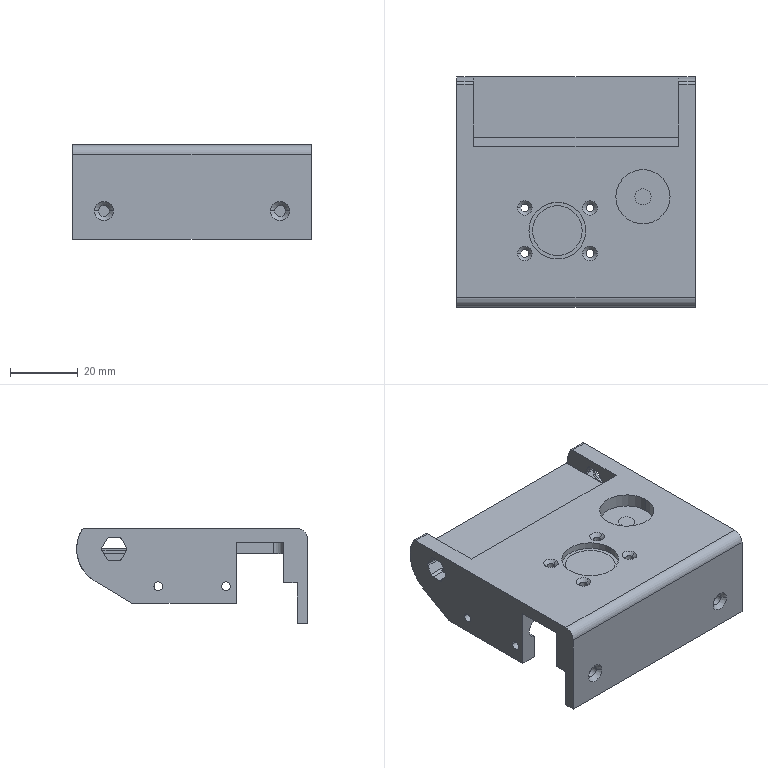NC program | NX | posted with a generic post | part box 70.5 x 68.1 x 28 mm
Whole program:
N10 G17 G21 G94 G90
(FLOOR_WALL_1_COPY_1 , TOOL : D10JING)
N12 T11 M6
N14 G54
N16 G17 G0 G90 X-13.5 Y24.372 B0. C0. S9500 M3
N18 G43 Z90. H11
N20 Z51.
N22 G94 G1 Z50. F1250.
N24 X-12.933 Y24.999
N26 G3 X-12.5 Y24.749 R0.5
N28 G1 X-0.833
N30 Y19.799
N32 X-12.5
N34 Y14.849
N36 X-0.833
N38 Y9.899
N40 X-12.5
N42 Y4.949
N44 X-0.833
N46 Y0.
N48 X-12.5
N50 Y-4.95
N52 X-0.833
N54 Y-9.9
N56 X-12.5
N58 Y-14.85
N60 X-0.833
N62 Y-19.8
N64 X-12.5
N66 Y-24.75
N68 X-0.833
N70 G3 X0.033 Y-24.25 R1.
N72 G1 X0.167 Y-24.018
N74 Z51.
N76 G0 Z90.
N78 X-13.595 Y-24.354
N80 Z51.
N82 G1 Z50.
N84 X-13.366 Y-24.75
N86 G3 X-12.5 Y-25.25 R1.
N88 G1 X-8.895
N90 X-0.833
N92 G3 X0.033 Y-24.75 R1.
N94 G1 X0.321 Y-24.25
N96 Z51.
N98 G0 Z90.
N100 Y24.25
N102 Z51.
N104 G1 Z50.
N106 X0.033 Y24.75
N108 G3 X-0.833 Y25.25 R1.
N110 G1 X-8.896
N112 X-12.5
N114 G3 X-13.366 Y24.75 R1.
N116 G1 X-13.595 Y24.354
N118 Z51.
N120 G0 Z90.
N122 M5
N124 M2